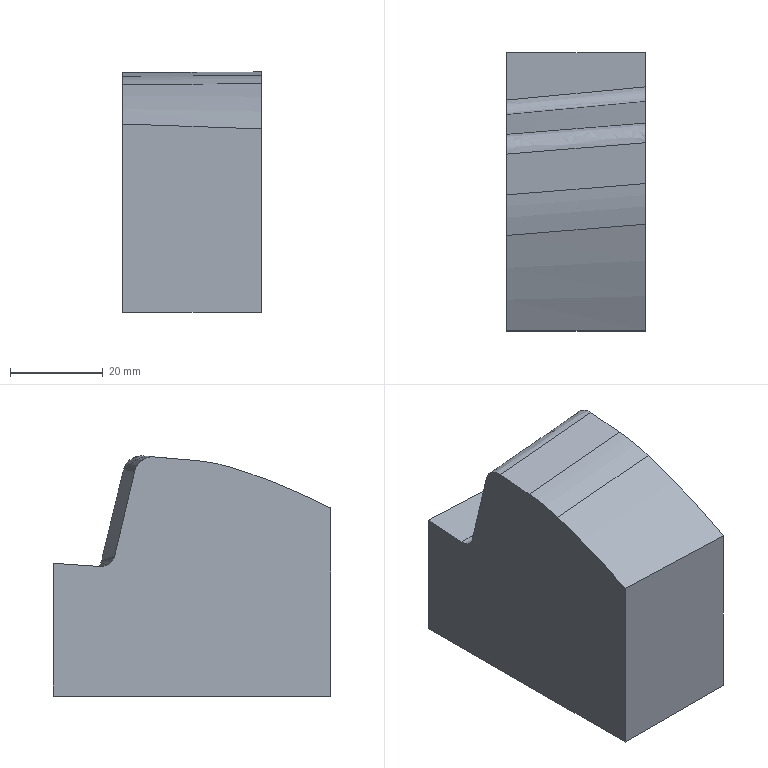Part | NX | features solid 2 | 1 solid | 12 faces | box 30 x 60 x 51.852 mm | volume 77898 mm3 | plane 7 | spline 4 | cylinder 1 | commonest cylinder face diameters 80 x1
STEP:
#1=CARTESIAN_POINT('',(635.,-588.785,-64.395));
#2=VERTEX_POINT('',#1);
#3=CARTESIAN_POINT('',(665.,-588.785,-65.46));
#4=VERTEX_POINT('',#3);
#5=CARTESIAN_POINT('',(635.,-588.785,-64.395));
#6=CARTESIAN_POINT('',(645.,-588.785,-64.74));
#7=CARTESIAN_POINT('',(655.,-588.785,-65.095));
#8=CARTESIAN_POINT('',(665.,-588.785,-65.46));
#9=B_SPLINE_CURVE_WITH_KNOTS('',3,(#5,#6,#7,#8),.UNSPECIFIED.,.F.,.F.,(4,4),(0.,0.03002),.UNSPECIFIED.);
#10=EDGE_CURVE('',#2,#4,#9,.T.);
#11=ORIENTED_EDGE('',*,*,#10,.F.);
#12=CARTESIAN_POINT('',(635.,-588.785,-105.));
#13=VERTEX_POINT('',#12);
#14=CARTESIAN_POINT('',(635.,-588.785,-115.));
#15=DIRECTION('',(0.,0.,1.));
#16=VECTOR('',#15,1000.);
#17=LINE('',#14,#16);
#18=EDGE_CURVE('',#13,#2,#17,.T.);
#19=ORIENTED_EDGE('',*,*,#18,.F.);
#20=CARTESIAN_POINT('',(665.,-588.785,-105.));
#21=VERTEX_POINT('',#20);
#22=CARTESIAN_POINT('',(675.,-588.785,-105.));
#23=DIRECTION('',(1.,0.,0.));
#24=VECTOR('',#23,1000.);
#25=LINE('',#22,#24);
#26=EDGE_CURVE('',#21,#13,#25,.F.);
#27=ORIENTED_EDGE('',*,*,#26,.F.);
#28=CARTESIAN_POINT('',(665.,-588.785,-115.));
#29=DIRECTION('',(0.,0.,-1.));
#30=VECTOR('',#29,1000.);
#31=LINE('',#28,#30);
#32=EDGE_CURVE('',#21,#4,#31,.F.);
#33=ORIENTED_EDGE('',*,*,#32,.T.);
#34=EDGE_LOOP('',(#11,#19,#27,#33));
#35=FACE_BOUND('',#34,.T.);
#36=CARTESIAN_POINT('',(675.,-588.785,-115.));
#37=DIRECTION('',(0.,-1.,0.));
#38=DIRECTION('',(-1.,0.,0.));
#39=AXIS2_PLACEMENT_3D('',#36,#37,#38);
#40=PLANE('',#39);
#41=ADVANCED_FACE('',(#35),#40,.T.);
#42=CARTESIAN_POINT('',(635.,-568.231,-55.911));
#43=VERTEX_POINT('',#42);
#44=CARTESIAN_POINT('',(635.,-568.231,-55.911));
#45=CARTESIAN_POINT('',(635.,-575.314,-58.178));
#46=CARTESIAN_POINT('',(635.,-582.165,-61.006));
#47=CARTESIAN_POINT('',(635.,-588.785,-64.395));
#48=B_SPLINE_CURVE_WITH_KNOTS('',3,(#44,#45,#46,#47),.UNSPECIFIED.,.F.,.F.,(4,4),(0.000006564,0.02224),.UNSPECIFIED.);
#49=EDGE_CURVE('',#43,#2,#48,.T.);
#50=ORIENTED_EDGE('',*,*,#49,.F.);
#51=CARTESIAN_POINT('',(635.,-559.467,-54.148));
#52=VERTEX_POINT('',#51);
#53=CARTESIAN_POINT('',(635.,-555.981,-93.996));
#54=DIRECTION('',(-1.,0.,0.));
#55=DIRECTION('',(0.,0.9962,0.08716));
#56=AXIS2_PLACEMENT_3D('',#53,#54,#55);
#57=ELLIPSE('',#56,40.132,40.);
#58=EDGE_CURVE('',#43,#52,#57,.T.);
#59=ORIENTED_EDGE('',*,*,#58,.T.);
#60=CARTESIAN_POINT('',(635.,-550.666,-53.378));
#61=VERTEX_POINT('',#60);
#62=CARTESIAN_POINT('',(635.,-573.997,-55.419));
#63=DIRECTION('',(0.,0.9962,0.08716));
#64=VECTOR('',#63,1000.);
#65=LINE('',#62,#64);
#66=EDGE_CURVE('',#61,#52,#65,.F.);
#67=ORIENTED_EDGE('',*,*,#66,.F.);
#68=CARTESIAN_POINT('',(635.,-546.41,-56.449));
#69=VERTEX_POINT('',#68);
#70=CARTESIAN_POINT('',(635.,-546.41,-56.449));
#71=CARTESIAN_POINT('',(635.,-546.63,-55.512));
#72=CARTESIAN_POINT('',(635.,-547.762,-53.838));
#73=CARTESIAN_POINT('',(635.,-549.708,-53.294));
#74=CARTESIAN_POINT('',(635.,-550.667,-53.378));
#75=B_SPLINE_CURVE_WITH_KNOTS('',3,(#70,#71,#72,#73,#74),.UNSPECIFIED.,.F.,.F.,(4,1,4),(0.,0.002846,0.005692),.UNSPECIFIED.);
#76=EDGE_CURVE('',#69,#61,#75,.T.);
#77=ORIENTED_EDGE('',*,*,#76,.F.);
#78=CARTESIAN_POINT('',(635.,-542.118,-74.723));
#79=VERTEX_POINT('',#78);
#80=CARTESIAN_POINT('',(635.,-542.118,-74.723));
#81=CARTESIAN_POINT('',(635.,-543.549,-68.632));
#82=CARTESIAN_POINT('',(635.,-544.98,-62.541));
#83=CARTESIAN_POINT('',(635.,-546.41,-56.449));
#84=B_SPLINE_CURVE_WITH_KNOTS('',3,(#80,#81,#82,#83),.UNSPECIFIED.,.F.,.F.,(4,4),(0.003708,0.02248),.UNSPECIFIED.);
#85=EDGE_CURVE('',#79,#69,#84,.T.);
#86=ORIENTED_EDGE('',*,*,#85,.F.);
#87=CARTESIAN_POINT('',(635.,-538.962,-77.044));
#88=VERTEX_POINT('',#87);
#89=CARTESIAN_POINT('',(635.,-542.118,-74.723));
#90=CARTESIAN_POINT('',(635.,-541.79,-76.119));
#91=CARTESIAN_POINT('',(635.,-540.392,-77.144));
#92=CARTESIAN_POINT('',(635.,-538.962,-77.044));
#93=B_SPLINE_CURVE_WITH_KNOTS('',3,(#89,#90,#91,#92),.UNSPECIFIED.,.F.,.F.,(4,4),(0.,0.004238),.UNSPECIFIED.);
#94=EDGE_CURVE('',#79,#88,#93,.T.);
#95=ORIENTED_EDGE('',*,*,#94,.T.);
#96=CARTESIAN_POINT('',(635.,-528.785,-76.332));
#97=VERTEX_POINT('',#96);
#98=CARTESIAN_POINT('',(635.,-571.281,-79.303));
#99=DIRECTION('',(0.,0.9976,0.06976));
#100=VECTOR('',#99,1000.);
#101=LINE('',#98,#100);
#102=EDGE_CURVE('',#97,#88,#101,.F.);
#103=ORIENTED_EDGE('',*,*,#102,.F.);
#104=CARTESIAN_POINT('',(635.,-528.785,-105.));
#105=VERTEX_POINT('',#104);
#106=CARTESIAN_POINT('',(635.,-528.785,-115.));
#107=DIRECTION('',(0.,0.,-1.));
#108=VECTOR('',#107,1000.);
#109=LINE('',#106,#108);
#110=EDGE_CURVE('',#105,#97,#109,.F.);
#111=ORIENTED_EDGE('',*,*,#110,.F.);
#112=CARTESIAN_POINT('',(635.,-568.785,-105.));
#113=DIRECTION('',(0.,-1.,0.));
#114=VECTOR('',#113,1000.);
#115=LINE('',#112,#114);
#116=EDGE_CURVE('',#13,#105,#115,.F.);
#117=ORIENTED_EDGE('',*,*,#116,.F.);
#118=ORIENTED_EDGE('',*,*,#18,.T.);
#119=EDGE_LOOP('',(#50,#59,#67,#77,#86,#95,#103,#111,#117,#118));
#120=FACE_BOUND('',#119,.T.);
#121=CARTESIAN_POINT('',(635.,-568.785,-115.));
#122=DIRECTION('',(-1.,0.,0.));
#123=DIRECTION('',(0.,1.,0.));
#124=AXIS2_PLACEMENT_3D('',#121,#122,#123);
#125=PLANE('',#124);
#126=ADVANCED_FACE('',(#120),#125,.T.);
#127=CARTESIAN_POINT('',(665.,-528.785,-77.645));
#128=VERTEX_POINT('',#127);
#129=CARTESIAN_POINT('',(676.612,-528.785,-78.153));
#130=DIRECTION('',(-0.999,0.,0.04372));
#131=VECTOR('',#130,1000.);
#132=LINE('',#129,#131);
#133=EDGE_CURVE('',#128,#97,#132,.T.);
#134=ORIENTED_EDGE('',*,*,#133,.F.);
#135=CARTESIAN_POINT('',(665.,-528.785,-105.));
#136=VERTEX_POINT('',#135);
#137=CARTESIAN_POINT('',(665.,-528.785,-115.));
#138=DIRECTION('',(0.,0.,1.));
#139=VECTOR('',#138,1000.);
#140=LINE('',#137,#139);
#141=EDGE_CURVE('',#136,#128,#140,.T.);
#142=ORIENTED_EDGE('',*,*,#141,.F.);
#143=CARTESIAN_POINT('',(675.,-528.785,-105.));
#144=DIRECTION('',(-1.,0.,0.));
#145=VECTOR('',#144,1000.);
#146=LINE('',#143,#145);
#147=EDGE_CURVE('',#136,#105,#146,.T.);
#148=ORIENTED_EDGE('',*,*,#147,.T.);
#149=ORIENTED_EDGE('',*,*,#110,.T.);
#150=EDGE_LOOP('',(#134,#142,#148,#149));
#151=FACE_BOUND('',#150,.T.);
#152=CARTESIAN_POINT('',(675.,-528.785,-115.));
#153=DIRECTION('',(0.,-1.,0.));
#154=DIRECTION('',(-1.,0.,0.));
#155=AXIS2_PLACEMENT_3D('',#152,#153,#154);
#156=PLANE('',#155);
#157=ADVANCED_FACE('',(#151),#156,.F.);
#158=CARTESIAN_POINT('',(665.,-565.797,-55.698));
#159=VERTEX_POINT('',#158);
#160=CARTESIAN_POINT('',(665.,-588.785,-65.46));
#161=CARTESIAN_POINT('',(665.,-581.422,-61.5));
#162=CARTESIAN_POINT('',(665.,-573.759,-58.246));
#163=CARTESIAN_POINT('',(665.,-565.797,-55.698));
#164=B_SPLINE_CURVE_WITH_KNOTS('',3,(#160,#161,#162,#163),.UNSPECIFIED.,.F.,.F.,(4,4),(0.,0.02497),.UNSPECIFIED.);
#165=EDGE_CURVE('',#4,#159,#164,.T.);
#166=ORIENTED_EDGE('',*,*,#165,.F.);
#167=ORIENTED_EDGE('',*,*,#32,.F.);
#168=CARTESIAN_POINT('',(665.,-568.785,-105.));
#169=DIRECTION('',(0.,1.,0.));
#170=VECTOR('',#169,1000.);
#171=LINE('',#168,#170);
#172=EDGE_CURVE('',#21,#136,#171,.T.);
#173=ORIENTED_EDGE('',*,*,#172,.T.);
#174=ORIENTED_EDGE('',*,*,#141,.T.);
#175=CARTESIAN_POINT('',(665.,-536.105,-78.157));
#176=VERTEX_POINT('',#175);
#177=CARTESIAN_POINT('',(665.,-571.19,-80.61));
#178=DIRECTION('',(0.,0.9976,0.06976));
#179=VECTOR('',#178,1000.);
#180=LINE('',#177,#179);
#181=EDGE_CURVE('',#176,#128,#180,.T.);
#182=ORIENTED_EDGE('',*,*,#181,.F.);
#183=CARTESIAN_POINT('',(665.,-539.258,-75.85));
#184=VERTEX_POINT('',#183);
#185=CARTESIAN_POINT('',(665.,-536.105,-78.157));
#186=CARTESIAN_POINT('',(665.,-537.531,-78.256));
#187=CARTESIAN_POINT('',(665.,-538.925,-77.239));
#188=CARTESIAN_POINT('',(665.,-539.258,-75.85));
#189=B_SPLINE_CURVE_WITH_KNOTS('',3,(#185,#186,#187,#188),.UNSPECIFIED.,.F.,.F.,(4,4),(0.,0.004226),.UNSPECIFIED.);
#190=EDGE_CURVE('',#176,#184,#189,.T.);
#191=ORIENTED_EDGE('',*,*,#190,.T.);
#192=CARTESIAN_POINT('',(665.,-543.963,-56.217));
#193=VERTEX_POINT('',#192);
#194=CARTESIAN_POINT('',(665.,-543.963,-56.217));
#195=CARTESIAN_POINT('',(665.,-542.395,-62.761));
#196=CARTESIAN_POINT('',(665.,-540.827,-69.306));
#197=CARTESIAN_POINT('',(665.,-539.258,-75.85));
#198=B_SPLINE_CURVE_WITH_KNOTS('',3,(#194,#195,#196,#197),.UNSPECIFIED.,.F.,.F.,(4,4),(0.002161,0.02235),.UNSPECIFIED.);
#199=EDGE_CURVE('',#193,#184,#198,.T.);
#200=ORIENTED_EDGE('',*,*,#199,.F.);
#201=CARTESIAN_POINT('',(665.,-548.214,-53.163));
#202=VERTEX_POINT('',#201);
#203=CARTESIAN_POINT('',(665.,-548.215,-53.163));
#204=CARTESIAN_POINT('',(665.,-547.26,-53.08));
#205=CARTESIAN_POINT('',(665.,-545.321,-53.619));
#206=CARTESIAN_POINT('',(665.,-544.186,-55.284));
#207=CARTESIAN_POINT('',(665.,-543.963,-56.217));
#208=B_SPLINE_CURVE_WITH_KNOTS('',3,(#203,#204,#205,#206,#207),.UNSPECIFIED.,.F.,.F.,(4,1,4),(0.,0.002837,0.005675),.UNSPECIFIED.);
#209=EDGE_CURVE('',#202,#193,#208,.T.);
#210=ORIENTED_EDGE('',*,*,#209,.F.);
#211=CARTESIAN_POINT('',(665.,-557.033,-53.935));
#212=VERTEX_POINT('',#211);
#213=CARTESIAN_POINT('',(665.,-573.997,-55.419));
#214=DIRECTION('',(0.,0.9962,0.08716));
#215=VECTOR('',#214,1000.);
#216=LINE('',#213,#215);
#217=EDGE_CURVE('',#212,#202,#216,.T.);
#218=ORIENTED_EDGE('',*,*,#217,.F.);
#219=CARTESIAN_POINT('',(665.,-553.547,-93.783));
#220=DIRECTION('',(-1.,0.,0.));
#221=DIRECTION('',(0.,0.9962,0.08716));
#222=AXIS2_PLACEMENT_3D('',#219,#220,#221);
#223=ELLIPSE('',#222,40.132,40.);
#224=EDGE_CURVE('',#212,#159,#223,.F.);
#225=ORIENTED_EDGE('',*,*,#224,.T.);
#226=EDGE_LOOP('',(#166,#167,#173,#174,#182,#191,#200,#210,#218,#225));
#227=FACE_BOUND('',#226,.T.);
#228=CARTESIAN_POINT('',(665.,-568.785,-115.));
#229=DIRECTION('',(-1.,0.,0.));
#230=DIRECTION('',(0.,1.,0.));
#231=AXIS2_PLACEMENT_3D('',#228,#229,#230);
#232=PLANE('',#231);
#233=ADVANCED_FACE('',(#227),#232,.F.);
#234=ORIENTED_EDGE('',*,*,#147,.F.);
#235=ORIENTED_EDGE('',*,*,#172,.F.);
#236=ORIENTED_EDGE('',*,*,#26,.T.);
#237=ORIENTED_EDGE('',*,*,#116,.T.);
#238=EDGE_LOOP('',(#234,#235,#236,#237));
#239=FACE_BOUND('',#238,.T.);
#240=CARTESIAN_POINT('',(675.,-568.785,-105.));
#241=DIRECTION('',(0.,0.,-1.));
#242=DIRECTION('',(-1.,0.,0.));
#243=AXIS2_PLACEMENT_3D('',#240,#241,#242);
#244=PLANE('',#243);
#245=ADVANCED_FACE('',(#239),#244,.T.);
#246=CARTESIAN_POINT('',(635.,-568.231,-55.911));
#247=CARTESIAN_POINT('',(645.,-567.42,-55.84));
#248=CARTESIAN_POINT('',(655.,-566.608,-55.769));
#249=CARTESIAN_POINT('',(665.,-565.797,-55.698));
#250=B_SPLINE_CURVE_WITH_KNOTS('',3,(#246,#247,#248,#249),.UNSPECIFIED.,.F.,.F.,(4,4),(0.3841,0.5664),.UNSPECIFIED.);
#251=EDGE_CURVE('',#159,#43,#250,.F.);
#252=ORIENTED_EDGE('',*,*,#251,.T.);
#253=ORIENTED_EDGE('',*,*,#49,.T.);
#254=ORIENTED_EDGE('',*,*,#10,.T.);
#255=ORIENTED_EDGE('',*,*,#165,.T.);
#256=EDGE_LOOP('',(#252,#253,#254,#255));
#257=FACE_BOUND('',#256,.T.);
#258=CARTESIAN_POINT('',(667.135,-588.744,-65.516));
#259=CARTESIAN_POINT('',(635.027,-591.349,-65.744));
#260=CARTESIAN_POINT('',(666.508,-581.415,-61.541));
#261=CARTESIAN_POINT('',(634.401,-584.019,-61.768));
#262=CARTESIAN_POINT('',(665.856,-573.717,-58.249));
#263=CARTESIAN_POINT('',(633.749,-576.321,-58.477));
#264=CARTESIAN_POINT('',(665.19,-565.782,-55.697));
#265=CARTESIAN_POINT('',(633.083,-568.387,-55.924));
#266=B_SPLINE_SURFACE_WITH_KNOTS('',3,1,((#258,#259),(#260,#261),(#262,#263),(#264,#265)),.SURF_OF_LINEAR_EXTRUSION.,.F.,.F.,.F.,(4,4),(2,2),(0.6824,0.9999),(0.,1.),.PIECEWISE_BEZIER_KNOTS.);
#267=ADVANCED_FACE('',(#257),#266,.T.);
#268=ORIENTED_EDGE('',*,*,#58,.F.);
#269=ORIENTED_EDGE('',*,*,#251,.F.);
#270=ORIENTED_EDGE('',*,*,#224,.F.);
#271=CARTESIAN_POINT('',(635.,-559.467,-54.148));
#272=CARTESIAN_POINT('',(645.,-558.656,-54.077));
#273=CARTESIAN_POINT('',(655.,-557.844,-54.006));
#274=CARTESIAN_POINT('',(665.,-557.033,-53.935));
#275=B_SPLINE_CURVE_WITH_KNOTS('',3,(#271,#272,#273,#274),.UNSPECIFIED.,.F.,.F.,(4,4),(0.3884,0.5707),.UNSPECIFIED.);
#276=EDGE_CURVE('',#212,#52,#275,.F.);
#277=ORIENTED_EDGE('',*,*,#276,.T.);
#278=EDGE_LOOP('',(#268,#269,#270,#277));
#279=FACE_BOUND('',#278,.T.);
#280=CARTESIAN_POINT('',(659.135,-554.023,-93.824));
#281=DIRECTION('',(0.9967,0.08086,0.007075));
#282=DIRECTION('',(-0.08117,0.9929,0.08687));
#283=AXIS2_PLACEMENT_3D('',#280,#281,#282);
#284=CYLINDRICAL_SURFACE('',#283,40.);
#285=ADVANCED_FACE('',(#279),#284,.T.);
#286=CARTESIAN_POINT('',(665.,-548.213,-53.163));
#287=CARTESIAN_POINT('',(654.599,-549.064,-53.238));
#288=CARTESIAN_POINT('',(644.599,-549.881,-53.309));
#289=CARTESIAN_POINT('',(635.,-550.664,-53.378));
#290=B_SPLINE_CURVE_WITH_KNOTS('',3,(#286,#287,#288,#289),.UNSPECIFIED.,.F.,.F.,(4,4),(0.3894,0.5651),.UNSPECIFIED.);
#291=EDGE_CURVE('',#202,#61,#290,.T.);
#292=ORIENTED_EDGE('',*,*,#291,.T.);
#293=ORIENTED_EDGE('',*,*,#66,.T.);
#294=ORIENTED_EDGE('',*,*,#276,.F.);
#295=ORIENTED_EDGE('',*,*,#217,.T.);
#296=EDGE_LOOP('',(#292,#293,#294,#295));
#297=FACE_BOUND('',#296,.T.);
#298=CARTESIAN_POINT('',(-186.787,-208.835,-23.471));
#299=DIRECTION('',(0.,-0.08716,0.9962));
#300=DIRECTION('',(1.,0.,0.));
#301=AXIS2_PLACEMENT_3D('',#298,#299,#300);
#302=PLANE('',#301);
#303=ADVANCED_FACE('',(#297),#302,.T.);
#304=CARTESIAN_POINT('',(665.,-543.963,-56.217));
#305=CARTESIAN_POINT('',(655.,-544.78,-56.295));
#306=CARTESIAN_POINT('',(645.,-545.596,-56.373));
#307=CARTESIAN_POINT('',(635.,-546.41,-56.449));
#308=B_SPLINE_CURVE_WITH_KNOTS('',3,(#304,#305,#306,#307),.UNSPECIFIED.,.F.,.F.,(4,4),(0.4405,0.6186),.UNSPECIFIED.);
#309=EDGE_CURVE('',#193,#69,#308,.T.);
#310=ORIENTED_EDGE('',*,*,#309,.T.);
#311=ORIENTED_EDGE('',*,*,#76,.T.);
#312=ORIENTED_EDGE('',*,*,#291,.F.);
#313=ORIENTED_EDGE('',*,*,#209,.T.);
#314=EDGE_LOOP('',(#310,#311,#312,#313));
#315=FACE_BOUND('',#314,.T.);
#316=CARTESIAN_POINT('',(665.182,-543.948,-56.216));
#317=CARTESIAN_POINT('',(665.189,-544.08,-55.662));
#318=CARTESIAN_POINT('',(665.204,-544.31,-55.132));
#319=CARTESIAN_POINT('',(665.227,-544.633,-54.648));
#320=CARTESIAN_POINT('',(665.287,-545.436,-53.818));
#321=CARTESIAN_POINT('',(665.368,-546.475,-53.316));
#322=CARTESIAN_POINT('',(665.413,-547.034,-53.162));
#323=CARTESIAN_POINT('',(665.459,-547.609,-53.11));
#324=CARTESIAN_POINT('',(665.506,-548.174,-53.16));
#325=CARTESIAN_POINT('',(659.045,-544.45,-56.264));
#326=CARTESIAN_POINT('',(659.052,-544.581,-55.709));
#327=CARTESIAN_POINT('',(659.067,-544.811,-55.179));
#328=CARTESIAN_POINT('',(659.089,-545.134,-54.695));
#329=CARTESIAN_POINT('',(659.149,-545.937,-53.863));
#330=CARTESIAN_POINT('',(659.231,-546.977,-53.361));
#331=CARTESIAN_POINT('',(659.275,-547.536,-53.206));
#332=CARTESIAN_POINT('',(659.322,-548.111,-53.154));
#333=CARTESIAN_POINT('',(659.369,-548.677,-53.204));
#334=CARTESIAN_POINT('',(652.907,-544.951,-56.311));
#335=CARTESIAN_POINT('',(652.914,-545.082,-55.757));
#336=CARTESIAN_POINT('',(652.929,-545.312,-55.225));
#337=CARTESIAN_POINT('',(652.952,-545.635,-54.741));
#338=CARTESIAN_POINT('',(653.012,-546.438,-53.908));
#339=CARTESIAN_POINT('',(653.093,-547.478,-53.405));
#340=CARTESIAN_POINT('',(653.138,-548.038,-53.25));
#341=CARTESIAN_POINT('',(653.185,-548.613,-53.198));
#342=CARTESIAN_POINT('',(653.231,-549.179,-53.248));
#343=CARTESIAN_POINT('',(646.77,-545.452,-56.359));
#344=CARTESIAN_POINT('',(646.777,-545.583,-55.804));
#345=CARTESIAN_POINT('',(646.792,-545.812,-55.272));
#346=CARTESIAN_POINT('',(646.815,-546.135,-54.786));
#347=CARTESIAN_POINT('',(646.874,-546.938,-53.953));
#348=CARTESIAN_POINT('',(646.956,-547.978,-53.449));
#349=CARTESIAN_POINT('',(647.,-548.538,-53.294));
#350=CARTESIAN_POINT('',(647.047,-549.114,-53.242));
#351=CARTESIAN_POINT('',(647.094,-549.68,-53.292));
#352=CARTESIAN_POINT('',(640.633,-545.952,-56.406));
#353=CARTESIAN_POINT('',(640.639,-546.082,-55.85));
#354=CARTESIAN_POINT('',(640.654,-546.311,-55.318));
#355=CARTESIAN_POINT('',(640.677,-546.634,-54.832));
#356=CARTESIAN_POINT('',(640.737,-547.437,-53.998));
#357=CARTESIAN_POINT('',(640.818,-548.478,-53.493));
#358=CARTESIAN_POINT('',(640.863,-549.039,-53.338));
#359=CARTESIAN_POINT('',(640.909,-549.614,-53.286));
#360=CARTESIAN_POINT('',(640.956,-550.181,-53.335));
#361=CARTESIAN_POINT('',(634.495,-546.451,-56.453));
#362=CARTESIAN_POINT('',(634.502,-546.581,-55.897));
#363=CARTESIAN_POINT('',(634.517,-546.81,-55.364));
#364=CARTESIAN_POINT('',(634.539,-547.133,-54.878));
#365=CARTESIAN_POINT('',(634.599,-547.936,-54.042));
#366=CARTESIAN_POINT('',(634.68,-548.978,-53.537));
#367=CARTESIAN_POINT('',(634.725,-549.538,-53.381));
#368=CARTESIAN_POINT('',(634.771,-550.114,-53.33));
#369=CARTESIAN_POINT('',(634.818,-550.681,-53.379));
#370=B_SPLINE_SURFACE_WITH_KNOTS('',5,5,((#316,#317,#318,#319,#320,#321,#322,#323,#324),(#325,#326,#327,#328,#329,#330,#331,#332,#333),(#334,#335,#336,#337,#338,#339,#340,#341,#342),(#343,#344,#345,#346,#347,#348,#349,#350,#351),(#352,#353,#354,#355,#356,#357,#358,#359,#360),(#361,#362,#363,#364,#365,#366,#367,#368,#369)),.UNSPECIFIED.,.F.,.F.,.F.,(6,6),(6,3,6),(0.4395,0.6216),(0.,0.5,1.),.UNSPECIFIED.);
#371=ADVANCED_FACE('',(#315),#370,.T.);
#372=CARTESIAN_POINT('',(665.,-539.258,-75.85));
#373=CARTESIAN_POINT('',(655.001,-540.219,-75.474));
#374=CARTESIAN_POINT('',(645.001,-541.172,-75.099));
#375=CARTESIAN_POINT('',(635.,-542.118,-74.723));
#376=B_SPLINE_CURVE_WITH_KNOTS('',3,(#372,#373,#374,#375),.UNSPECIFIED.,.F.,.F.,(4,4),(0.3363,0.5192),.UNSPECIFIED.);
#377=EDGE_CURVE('',#184,#79,#376,.T.);
#378=ORIENTED_EDGE('',*,*,#377,.T.);
#379=ORIENTED_EDGE('',*,*,#85,.T.);
#380=ORIENTED_EDGE('',*,*,#309,.F.);
#381=ORIENTED_EDGE('',*,*,#199,.T.);
#382=EDGE_LOOP('',(#378,#379,#380,#381));
#383=FACE_BOUND('',#382,.T.);
#384=CARTESIAN_POINT('',(665.18,-539.213,-75.971));
#385=CARTESIAN_POINT('',(665.421,-540.779,-69.353));
#386=CARTESIAN_POINT('',(665.663,-542.345,-62.735));
#387=CARTESIAN_POINT('',(665.904,-543.911,-56.117));
#388=CARTESIAN_POINT('',(658.969,-539.783,-75.853));
#389=CARTESIAN_POINT('',(659.211,-541.342,-69.234));
#390=CARTESIAN_POINT('',(659.452,-542.901,-62.614));
#391=CARTESIAN_POINT('',(659.694,-544.46,-55.995));
#392=CARTESIAN_POINT('',(652.758,-540.35,-75.736));
#393=CARTESIAN_POINT('',(653.,-541.902,-69.115));
#394=CARTESIAN_POINT('',(653.241,-543.455,-62.494));
#395=CARTESIAN_POINT('',(653.483,-545.007,-55.873));
#396=CARTESIAN_POINT('',(646.547,-540.914,-75.619));
#397=CARTESIAN_POINT('',(646.789,-542.461,-68.997));
#398=CARTESIAN_POINT('',(647.03,-544.007,-62.375));
#399=CARTESIAN_POINT('',(647.272,-545.554,-55.752));
#400=CARTESIAN_POINT('',(640.336,-541.477,-75.503));
#401=CARTESIAN_POINT('',(640.577,-543.018,-68.879));
#402=CARTESIAN_POINT('',(640.819,-544.558,-62.255));
#403=CARTESIAN_POINT('',(641.061,-546.099,-55.631));
#404=CARTESIAN_POINT('',(634.124,-542.037,-75.386));
#405=CARTESIAN_POINT('',(634.366,-543.572,-68.761));
#406=CARTESIAN_POINT('',(634.608,-545.108,-62.136));
#407=CARTESIAN_POINT('',(634.85,-546.643,-55.511));
#408=B_SPLINE_SURFACE_WITH_KNOTS('',5,3,((#384,#385,#386,#387),(#388,#389,#390,#391),(#392,#393,#394,#395),(#396,#397,#398,#399),(#400,#401,#402,#403),(#404,#405,#406,#407)),.UNSPECIFIED.,.F.,.F.,.F.,(6,6),(4,4),(0.4026,0.5721),(0.1181,0.9199),.PIECEWISE_BEZIER_KNOTS.);
#409=ADVANCED_FACE('',(#383),#408,.T.);
#410=ORIENTED_EDGE('',*,*,#94,.F.);
#411=ORIENTED_EDGE('',*,*,#377,.F.);
#412=ORIENTED_EDGE('',*,*,#190,.F.);
#413=CARTESIAN_POINT('',(635.,-538.962,-77.044));
#414=CARTESIAN_POINT('',(645.075,-538.01,-77.418));
#415=CARTESIAN_POINT('',(655.075,-537.058,-77.789));
#416=CARTESIAN_POINT('',(665.,-536.105,-78.157));
#417=B_SPLINE_CURVE_WITH_KNOTS('',3,(#413,#414,#415,#416),.UNSPECIFIED.,.F.,.F.,(4,4),(0.4731,0.657),.UNSPECIFIED.);
#418=EDGE_CURVE('',#88,#176,#417,.T.);
#419=ORIENTED_EDGE('',*,*,#418,.F.);
#420=EDGE_LOOP('',(#410,#411,#412,#419));
#421=FACE_BOUND('',#420,.T.);
#422=CARTESIAN_POINT('',(634.437,-539.016,-77.023));
#423=CARTESIAN_POINT('',(634.476,-539.437,-77.054));
#424=CARTESIAN_POINT('',(634.518,-539.864,-77.01));
#425=CARTESIAN_POINT('',(634.561,-540.278,-76.891));
#426=CARTESIAN_POINT('',(634.648,-541.046,-76.509));
#427=CARTESIAN_POINT('',(634.727,-541.636,-75.887));
#428=CARTESIAN_POINT('',(634.763,-541.872,-75.525));
#429=CARTESIAN_POINT('',(634.793,-542.04,-75.129));
#430=CARTESIAN_POINT('',(634.818,-542.135,-74.717));
#431=CARTESIAN_POINT('',(635.104,-538.953,-77.047));
#432=CARTESIAN_POINT('',(635.142,-539.374,-77.079));
#433=CARTESIAN_POINT('',(635.184,-539.801,-77.035));
#434=CARTESIAN_POINT('',(635.228,-540.215,-76.915));
#435=CARTESIAN_POINT('',(635.314,-540.983,-76.534));
#436=CARTESIAN_POINT('',(635.393,-541.573,-75.911));
#437=CARTESIAN_POINT('',(635.429,-541.809,-75.55));
#438=CARTESIAN_POINT('',(635.46,-541.977,-75.154));
#439=CARTESIAN_POINT('',(635.484,-542.072,-74.742));
#440=CARTESIAN_POINT('',(635.77,-538.89,-77.072));
#441=CARTESIAN_POINT('',(635.809,-539.311,-77.103));
#442=CARTESIAN_POINT('',(635.85,-539.738,-77.06));
#443=CARTESIAN_POINT('',(635.894,-540.152,-76.94));
#444=CARTESIAN_POINT('',(635.981,-540.92,-76.559));
#445=CARTESIAN_POINT('',(636.06,-541.51,-75.936));
#446=CARTESIAN_POINT('',(636.095,-541.746,-75.575));
#447=CARTESIAN_POINT('',(636.126,-541.914,-75.179));
#448=CARTESIAN_POINT('',(636.15,-542.009,-74.767));
#449=CARTESIAN_POINT('',(636.436,-538.827,-77.097));
#450=CARTESIAN_POINT('',(636.475,-539.248,-77.128));
#451=CARTESIAN_POINT('',(636.517,-539.675,-77.084));
#452=CARTESIAN_POINT('',(636.56,-540.089,-76.965));
#453=CARTESIAN_POINT('',(636.647,-540.856,-76.584));
#454=CARTESIAN_POINT('',(636.726,-541.447,-75.961));
#455=CARTESIAN_POINT('',(636.762,-541.683,-75.6));
#456=CARTESIAN_POINT('',(636.792,-541.851,-75.204));
#457=CARTESIAN_POINT('',(636.817,-541.946,-74.792));
#458=CARTESIAN_POINT('',(642.585,-538.245,-77.325));
#459=CARTESIAN_POINT('',(642.624,-538.666,-77.356));
#460=CARTESIAN_POINT('',(642.666,-539.092,-77.313));
#461=CARTESIAN_POINT('',(642.71,-539.506,-77.194));
#462=CARTESIAN_POINT('',(642.797,-540.274,-76.813));
#463=CARTESIAN_POINT('',(642.876,-540.864,-76.191));
#464=CARTESIAN_POINT('',(642.912,-541.101,-75.83));
#465=CARTESIAN_POINT('',(642.942,-541.268,-75.435));
#466=CARTESIAN_POINT('',(642.967,-541.364,-75.022));
#467=CARTESIAN_POINT('',(648.735,-537.661,-77.554));
#468=CARTESIAN_POINT('',(648.773,-538.082,-77.585));
#469=CARTESIAN_POINT('',(648.816,-538.508,-77.541));
#470=CARTESIAN_POINT('',(648.859,-538.922,-77.422));
#471=CARTESIAN_POINT('',(648.946,-539.689,-77.042));
#472=CARTESIAN_POINT('',(649.026,-540.279,-76.421));
#473=CARTESIAN_POINT('',(649.062,-540.515,-76.06));
#474=CARTESIAN_POINT('',(649.092,-540.684,-75.665));
#475=CARTESIAN_POINT('',(649.117,-540.779,-75.253));
#476=CARTESIAN_POINT('',(654.217,-537.139,-77.757));
#477=CARTESIAN_POINT('',(654.256,-537.559,-77.788));
#478=CARTESIAN_POINT('',(654.299,-537.985,-77.745));
#479=CARTESIAN_POINT('',(654.342,-538.398,-77.626));
#480=CARTESIAN_POINT('',(654.43,-539.165,-77.246));
#481=CARTESIAN_POINT('',(654.509,-539.755,-76.626));
#482=CARTESIAN_POINT('',(654.545,-539.992,-76.265));
#483=CARTESIAN_POINT('',(654.576,-540.16,-75.871));
#484=CARTESIAN_POINT('',(654.6,-540.256,-75.459));
#485=CARTESIAN_POINT('',(659.7,-536.614,-77.96));
#486=CARTESIAN_POINT('',(659.739,-537.034,-77.991));
#487=CARTESIAN_POINT('',(659.781,-537.46,-77.948));
#488=CARTESIAN_POINT('',(659.825,-537.873,-77.829));
#489=CARTESIAN_POINT('',(659.913,-538.639,-77.45));
#490=CARTESIAN_POINT('',(659.992,-539.229,-76.83));
#491=CARTESIAN_POINT('',(660.028,-539.466,-76.47));
#492=CARTESIAN_POINT('',(660.059,-539.635,-76.076));
#493=CARTESIAN_POINT('',(660.083,-539.731,-75.665));
#494=CARTESIAN_POINT('',(665.182,-536.088,-78.163));
#495=CARTESIAN_POINT('',(665.221,-536.508,-78.194));
#496=CARTESIAN_POINT('',(665.264,-536.933,-78.151));
#497=CARTESIAN_POINT('',(665.308,-537.346,-78.032));
#498=CARTESIAN_POINT('',(665.395,-538.112,-77.654));
#499=CARTESIAN_POINT('',(665.475,-538.702,-77.035));
#500=CARTESIAN_POINT('',(665.511,-538.939,-76.676));
#501=CARTESIAN_POINT('',(665.542,-539.107,-76.282));
#502=CARTESIAN_POINT('',(665.566,-539.204,-75.871));
#503=B_SPLINE_SURFACE_WITH_KNOTS('',5,5,((#422,#423,#424,#425,#426,#427,#428,#429,#430),(#431,#432,#433,#434,#435,#436,#437,#438,#439),(#440,#441,#442,#443,#444,#445,#446,#447,#448),(#449,#450,#451,#452,#453,#454,#455,#456,#457),(#458,#459,#460,#461,#462,#463,#464,#465,#466),(#467,#468,#469,#470,#471,#472,#473,#474,#475),(#476,#477,#478,#479,#480,#481,#482,#483,#484),(#485,#486,#487,#488,#489,#490,#491,#492,#493),(#494,#495,#496,#497,#498,#499,#500,#501,#502)),.UNSPECIFIED.,.F.,.F.,.F.,(6,3,6),(6,3,6),(0.4797,0.5,0.6672),(0.,0.5,1.),.UNSPECIFIED.);
#504=ADVANCED_FACE('',(#421),#503,.F.);
#505=ORIENTED_EDGE('',*,*,#133,.T.);
#506=ORIENTED_EDGE('',*,*,#102,.T.);
#507=ORIENTED_EDGE('',*,*,#418,.T.);
#508=ORIENTED_EDGE('',*,*,#181,.T.);
#509=EDGE_LOOP('',(#505,#506,#507,#508));
#510=FACE_BOUND('',#509,.T.);
#511=CARTESIAN_POINT('',(405.253,-346.483,-53.53));
#512=DIRECTION('',(0.04361,-0.06969,0.9966));
#513=DIRECTION('',(0.999,0.003802,-0.04345));
#514=AXIS2_PLACEMENT_3D('',#511,#512,#513);
#515=PLANE('',#514);
#516=ADVANCED_FACE('',(#510),#515,.T.);
#517=CLOSED_SHELL('',(#41,#126,#157,#233,#245,#267,#285,#303,#371,#409,#504,#516));
#518=MANIFOLD_SOLID_BREP('',#517);
#519=(LENGTH_UNIT()NAMED_UNIT(*)SI_UNIT(.MILLI.,.METRE.));
#520=UNCERTAINTY_MEASURE_WITH_UNIT(LENGTH_MEASURE(0.0508),#519,'','');
#521=(NAMED_UNIT(*)PLANE_ANGLE_UNIT()SI_UNIT($,.RADIAN.));
#522=(NAMED_UNIT(*)SI_UNIT($,.STERADIAN.)SOLID_ANGLE_UNIT());
#523=(GEOMETRIC_REPRESENTATION_CONTEXT(3)GLOBAL_UNCERTAINTY_ASSIGNED_CONTEXT((#520))GLOBAL_UNIT_ASSIGNED_CONTEXT((#519,#521,#522))REPRESENTATION_CONTEXT('',''));
#524=ADVANCED_BREP_SHAPE_REPRESENTATION('',(#518),#523);